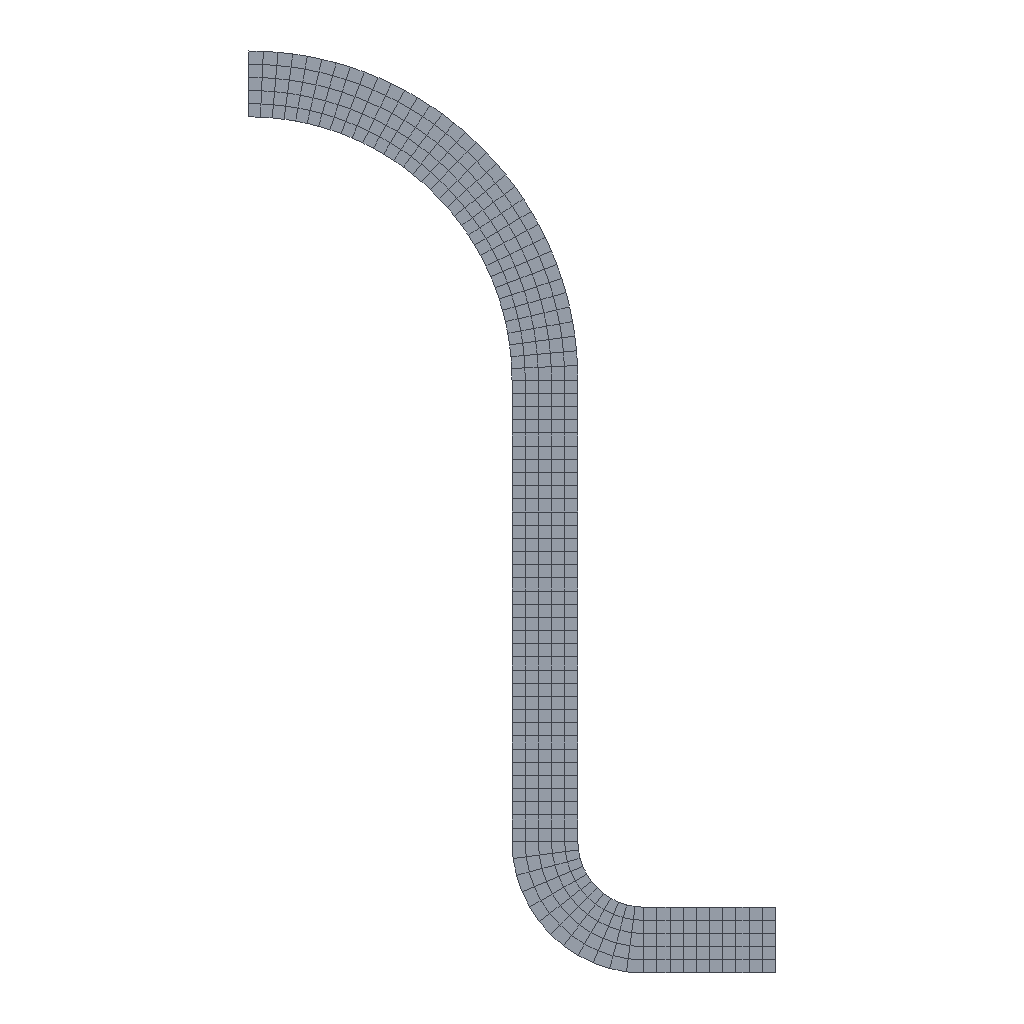Simulation study | abaqus
Set-up summary:
category,name,step,type,value,unit,region
solver,abaqus
solver,version,,,Abaqus/Standard 6.13-1
units,not stated in the deck,,not stated
analysis,deck,,static,static
load_step,Step-Static,Step-Static,static
load_step,requested,,,1
mesh,nodes,,,558
mesh,elements,,,460
element_type,CAX4R,,axisymmetric,460
load,load commands in deck,,count,1
bc,support commands in deck,,count,1
material,MAT-STEEL,,in results
check,setup vs results,,match,"per instance, exact: element labels, types and connectivity; labels of the nodes the elements use; coordinates of those nodes at SINGLE_PRECISION in 1 of 1 instance(s)"
Abaqus input file, long lists of numbers shortened:
*Heading
** Job name:  Model name: Model-1
** Generated by: Abaqus/CAE 6.13-1
*Preprint, echo=NO, model=NO, history=NO, contact=NO
**
** PARTS
**
*Part, name=Part-1
*Node
      1,         600.,         100.
      2,         600.,           0.
** (556 more lines like these left out)
*Element, type=CAX4R
 1,   1,  11, 207,  36
 2,  11,  12, 208, 207
** (458 more lines like these left out)
*Nset, nset=_PickedSet8, internal, generate
   1,  558,    1
*Elset, elset=_PickedSet8, internal, generate
   1,  460,    1
** Section: SectSt
*Solid Section, elset=_PickedSet8, material=Mat-Steel
,
*End Part
**
**
** ASSEMBLY
**
*Assembly, name=Assembly
**
*Instance, name=Part-1-1, part=Part-1
*End Instance
**
*Nset, nset=Set-Nds, instance=Part-1-1
  5,  8, 10
*Nset, nset=_PickedSet5, internal, instance=Part-1-1
  2,  3, 15, 16, 17, 18, 19, 20, 21, 22, 23
*Elset, elset=_PickedSet5, internal, instance=Part-1-1, generate
  5,  50,   5
*Elset, elset=__PickedSurf6_S4, internal, instance=Part-1-1, generate
  51,  456,    5
*Surface, type=ELEMENT, name=_PickedSurf6, internal
__PickedSurf6_S4, S4
*End Assembly
**
** MATERIALS
**
*Material, name=Mat-Steel
*Elastic
200000., 0.3
**
** BOUNDARY CONDITIONS
**
** Name: BC-1 Type: Symmetry/Antisymmetry/Encastre
*Boundary
_PickedSet5, ENCASTRE
** ----------------------------------------------------------------
**
** STEP: Step-Static
**
*Step, name=Step-Static, nlgeom=NO
*Static
0.01, 1., 1e-05, 0.05
**
** LOADS
**
** Name: Load-1   Type: Pressure
*Dsload
_PickedSurf6, P, 20.
**
** OUTPUT REQUESTS
**
*Restart, write, frequency=0
**
** FIELD OUTPUT: F-Output-1
**
*Output, field
*Node Output
U,
*Element Output, directions=YES
E, S
**
** HISTORY OUTPUT: H-Output-1
**
*Output, history
*Node Output, nset=Set-Nds
U1, U2
*End Step
Results summary:
result,step,Step-Static,completed,increments=24 time=1.0/1.0
result,analysis,,,static
result,last_loadstep,,,1
result,primary field,,,U